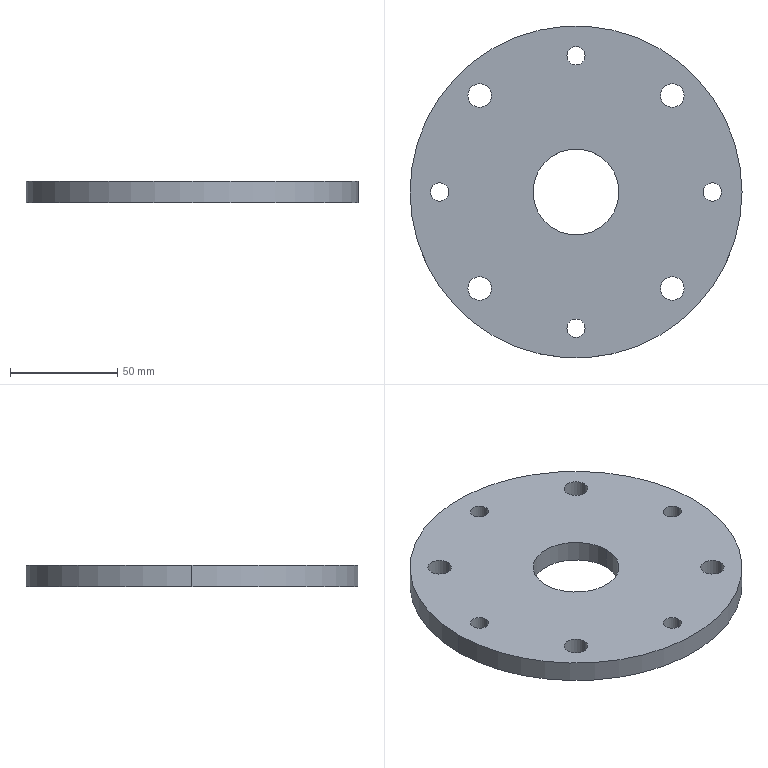Part | SolidWorks | features BaseBody 1, ICE 1 | 1 solid | 22 faces | box 155 x 155 x 10 mm | volume 169991 mm3 | cylinder 20 | plane 2 | commonest cylinder face diameters 8.5 x8 11 x8 40.1 x2 155 x2
STEP:
#1=CARTESIAN_POINT('',(20.05,0.,0.));
#2=VERTEX_POINT('',#1);
#3=CARTESIAN_POINT('',(-20.05,0.,0.));
#4=VERTEX_POINT('',#3);
#5=CARTESIAN_POINT('',(0.,0.,0.));
#6=DIRECTION('',(0.,0.,-1.));
#7=DIRECTION('',(0.,-1.,0.));
#8=AXIS2_PLACEMENT_3D('',#5,#6,#7);
#9=CIRCLE('',#8,20.05);
#10=EDGE_CURVE('',#2,#4,#9,.T.);
#11=ORIENTED_EDGE('',*,*,#10,.T.);
#12=CARTESIAN_POINT('',(-20.05,0.,10.));
#13=VERTEX_POINT('',#12);
#14=CARTESIAN_POINT('',(-20.05,0.,-0.001));
#15=DIRECTION('',(0.,0.,1.));
#16=VECTOR('',#15,1000.);
#17=LINE('',#14,#16);
#18=EDGE_CURVE('',#4,#13,#17,.T.);
#19=ORIENTED_EDGE('',*,*,#18,.T.);
#20=CARTESIAN_POINT('',(20.05,0.,10.));
#21=VERTEX_POINT('',#20);
#22=CARTESIAN_POINT('',(0.,0.,10.));
#23=DIRECTION('',(0.,0.,1.));
#24=DIRECTION('',(1.,0.,0.));
#25=AXIS2_PLACEMENT_3D('',#22,#23,#24);
#26=CIRCLE('',#25,20.05);
#27=EDGE_CURVE('',#13,#21,#26,.T.);
#28=ORIENTED_EDGE('',*,*,#27,.T.);
#29=CARTESIAN_POINT('',(20.05,0.,-0.001));
#30=DIRECTION('',(0.,0.,1.));
#31=VECTOR('',#30,1000.);
#32=LINE('',#29,#31);
#33=EDGE_CURVE('',#2,#21,#32,.T.);
#34=ORIENTED_EDGE('',*,*,#33,.F.);
#35=EDGE_LOOP('',(#11,#19,#28,#34));
#36=FACE_OUTER_BOUND('',#35,.T.);
#37=CARTESIAN_POINT('',(0.,0.,-0.001));
#38=DIRECTION('',(0.,0.,1.));
#39=DIRECTION('',(1.,0.,0.));
#40=AXIS2_PLACEMENT_3D('',#37,#38,#39);
#41=CYLINDRICAL_SURFACE('',#40,20.05);
#42=ADVANCED_FACE('',(#36),#41,.F.);
#43=CARTESIAN_POINT('',(-4.25,63.64,0.));
#44=VERTEX_POINT('',#43);
#45=CARTESIAN_POINT('',(4.25,63.64,0.));
#46=VERTEX_POINT('',#45);
#47=CARTESIAN_POINT('',(0.,63.64,0.));
#48=DIRECTION('',(0.,0.,1.));
#49=DIRECTION('',(1.,0.,0.));
#50=AXIS2_PLACEMENT_3D('',#47,#48,#49);
#51=CIRCLE('',#50,4.25);
#52=EDGE_CURVE('',#44,#46,#51,.T.);
#53=ORIENTED_EDGE('',*,*,#52,.F.);
#54=CARTESIAN_POINT('',(-4.25,63.64,10.));
#55=VERTEX_POINT('',#54);
#56=CARTESIAN_POINT('',(-4.25,63.64,10.));
#57=DIRECTION('',(0.,0.,1.));
#58=VECTOR('',#57,1000.);
#59=LINE('',#56,#58);
#60=EDGE_CURVE('',#44,#55,#59,.T.);
#61=ORIENTED_EDGE('',*,*,#60,.T.);
#62=CARTESIAN_POINT('',(4.25,63.64,10.));
#63=VERTEX_POINT('',#62);
#64=CARTESIAN_POINT('',(0.,63.64,10.));
#65=DIRECTION('',(0.,0.,1.));
#66=DIRECTION('',(1.,0.,0.));
#67=AXIS2_PLACEMENT_3D('',#64,#65,#66);
#68=CIRCLE('',#67,4.25);
#69=EDGE_CURVE('',#55,#63,#68,.T.);
#70=ORIENTED_EDGE('',*,*,#69,.T.);
#71=CARTESIAN_POINT('',(4.25,63.64,10.));
#72=DIRECTION('',(0.,0.,1.));
#73=VECTOR('',#72,1000.);
#74=LINE('',#71,#73);
#75=EDGE_CURVE('',#46,#63,#74,.T.);
#76=ORIENTED_EDGE('',*,*,#75,.F.);
#77=EDGE_LOOP('',(#53,#61,#70,#76));
#78=FACE_OUTER_BOUND('',#77,.T.);
#79=CARTESIAN_POINT('',(0.,63.64,10.));
#80=DIRECTION('',(0.,0.,1.));
#81=DIRECTION('',(1.,0.,0.));
#82=AXIS2_PLACEMENT_3D('',#79,#80,#81);
#83=CYLINDRICAL_SURFACE('',#82,4.25);
#84=ADVANCED_FACE('',(#78),#83,.F.);
#85=CARTESIAN_POINT('',(-67.89,0.,0.));
#86=VERTEX_POINT('',#85);
#87=CARTESIAN_POINT('',(-59.39,0.,0.));
#88=VERTEX_POINT('',#87);
#89=CARTESIAN_POINT('',(-63.64,0.,0.));
#90=DIRECTION('',(0.,0.,1.));
#91=DIRECTION('',(1.,0.,0.));
#92=AXIS2_PLACEMENT_3D('',#89,#90,#91);
#93=CIRCLE('',#92,4.25);
#94=EDGE_CURVE('',#86,#88,#93,.T.);
#95=ORIENTED_EDGE('',*,*,#94,.F.);
#96=CARTESIAN_POINT('',(-67.89,0.,10.));
#97=VERTEX_POINT('',#96);
#98=CARTESIAN_POINT('',(-67.89,0.,10.));
#99=DIRECTION('',(0.,0.,1.));
#100=VECTOR('',#99,1000.);
#101=LINE('',#98,#100);
#102=EDGE_CURVE('',#86,#97,#101,.T.);
#103=ORIENTED_EDGE('',*,*,#102,.T.);
#104=CARTESIAN_POINT('',(-59.39,0.,10.));
#105=VERTEX_POINT('',#104);
#106=CARTESIAN_POINT('',(-63.64,0.,10.));
#107=DIRECTION('',(0.,0.,1.));
#108=DIRECTION('',(1.,0.,0.));
#109=AXIS2_PLACEMENT_3D('',#106,#107,#108);
#110=CIRCLE('',#109,4.25);
#111=EDGE_CURVE('',#97,#105,#110,.T.);
#112=ORIENTED_EDGE('',*,*,#111,.T.);
#113=CARTESIAN_POINT('',(-59.39,0.,10.));
#114=DIRECTION('',(0.,0.,1.));
#115=VECTOR('',#114,1000.);
#116=LINE('',#113,#115);
#117=EDGE_CURVE('',#88,#105,#116,.T.);
#118=ORIENTED_EDGE('',*,*,#117,.F.);
#119=EDGE_LOOP('',(#95,#103,#112,#118));
#120=FACE_OUTER_BOUND('',#119,.T.);
#121=CARTESIAN_POINT('',(-63.64,0.,10.));
#122=DIRECTION('',(0.,0.,1.));
#123=DIRECTION('',(1.,0.,0.));
#124=AXIS2_PLACEMENT_3D('',#121,#122,#123);
#125=CYLINDRICAL_SURFACE('',#124,4.25);
#126=ADVANCED_FACE('',(#120),#125,.F.);
#127=CARTESIAN_POINT('',(-4.25,-63.64,0.));
#128=VERTEX_POINT('',#127);
#129=CARTESIAN_POINT('',(4.25,-63.64,0.));
#130=VERTEX_POINT('',#129);
#131=CARTESIAN_POINT('',(0.,-63.64,0.));
#132=DIRECTION('',(0.,0.,1.));
#133=DIRECTION('',(1.,0.,0.));
#134=AXIS2_PLACEMENT_3D('',#131,#132,#133);
#135=CIRCLE('',#134,4.25);
#136=EDGE_CURVE('',#128,#130,#135,.T.);
#137=ORIENTED_EDGE('',*,*,#136,.F.);
#138=CARTESIAN_POINT('',(-4.25,-63.64,10.));
#139=VERTEX_POINT('',#138);
#140=CARTESIAN_POINT('',(-4.25,-63.64,10.));
#141=DIRECTION('',(0.,0.,1.));
#142=VECTOR('',#141,1000.);
#143=LINE('',#140,#142);
#144=EDGE_CURVE('',#128,#139,#143,.T.);
#145=ORIENTED_EDGE('',*,*,#144,.T.);
#146=CARTESIAN_POINT('',(4.25,-63.64,10.));
#147=VERTEX_POINT('',#146);
#148=CARTESIAN_POINT('',(0.,-63.64,10.));
#149=DIRECTION('',(0.,0.,1.));
#150=DIRECTION('',(1.,0.,0.));
#151=AXIS2_PLACEMENT_3D('',#148,#149,#150);
#152=CIRCLE('',#151,4.25);
#153=EDGE_CURVE('',#139,#147,#152,.T.);
#154=ORIENTED_EDGE('',*,*,#153,.T.);
#155=CARTESIAN_POINT('',(4.25,-63.64,10.));
#156=DIRECTION('',(0.,0.,1.));
#157=VECTOR('',#156,1000.);
#158=LINE('',#155,#157);
#159=EDGE_CURVE('',#130,#147,#158,.T.);
#160=ORIENTED_EDGE('',*,*,#159,.F.);
#161=EDGE_LOOP('',(#137,#145,#154,#160));
#162=FACE_OUTER_BOUND('',#161,.T.);
#163=CARTESIAN_POINT('',(0.,-63.64,10.));
#164=DIRECTION('',(0.,0.,1.));
#165=DIRECTION('',(1.,0.,0.));
#166=AXIS2_PLACEMENT_3D('',#163,#164,#165);
#167=CYLINDRICAL_SURFACE('',#166,4.25);
#168=ADVANCED_FACE('',(#162),#167,.F.);
#169=CARTESIAN_POINT('',(59.39,0.,0.));
#170=VERTEX_POINT('',#169);
#171=CARTESIAN_POINT('',(67.89,0.,0.));
#172=VERTEX_POINT('',#171);
#173=CARTESIAN_POINT('',(63.64,0.,0.));
#174=DIRECTION('',(0.,0.,1.));
#175=DIRECTION('',(1.,0.,0.));
#176=AXIS2_PLACEMENT_3D('',#173,#174,#175);
#177=CIRCLE('',#176,4.25);
#178=EDGE_CURVE('',#170,#172,#177,.T.);
#179=ORIENTED_EDGE('',*,*,#178,.F.);
#180=CARTESIAN_POINT('',(59.39,0.,10.));
#181=VERTEX_POINT('',#180);
#182=CARTESIAN_POINT('',(59.39,0.,10.));
#183=DIRECTION('',(0.,0.,1.));
#184=VECTOR('',#183,1000.);
#185=LINE('',#182,#184);
#186=EDGE_CURVE('',#170,#181,#185,.T.);
#187=ORIENTED_EDGE('',*,*,#186,.T.);
#188=CARTESIAN_POINT('',(67.89,0.,10.));
#189=VERTEX_POINT('',#188);
#190=CARTESIAN_POINT('',(63.64,0.,10.));
#191=DIRECTION('',(0.,0.,1.));
#192=DIRECTION('',(1.,0.,0.));
#193=AXIS2_PLACEMENT_3D('',#190,#191,#192);
#194=CIRCLE('',#193,4.25);
#195=EDGE_CURVE('',#181,#189,#194,.T.);
#196=ORIENTED_EDGE('',*,*,#195,.T.);
#197=CARTESIAN_POINT('',(67.89,0.,10.));
#198=DIRECTION('',(0.,0.,1.));
#199=VECTOR('',#198,1000.);
#200=LINE('',#197,#199);
#201=EDGE_CURVE('',#172,#189,#200,.T.);
#202=ORIENTED_EDGE('',*,*,#201,.F.);
#203=EDGE_LOOP('',(#179,#187,#196,#202));
#204=FACE_OUTER_BOUND('',#203,.T.);
#205=CARTESIAN_POINT('',(63.64,0.,10.));
#206=DIRECTION('',(0.,0.,1.));
#207=DIRECTION('',(1.,0.,0.));
#208=AXIS2_PLACEMENT_3D('',#205,#206,#207);
#209=CYLINDRICAL_SURFACE('',#208,4.25);
#210=ADVANCED_FACE('',(#204),#209,.F.);
#211=CARTESIAN_POINT('',(-50.5,45.,0.));
#212=VERTEX_POINT('',#211);
#213=CARTESIAN_POINT('',(-39.5,45.,0.));
#214=VERTEX_POINT('',#213);
#215=CARTESIAN_POINT('',(-45.,45.,0.));
#216=DIRECTION('',(0.,0.,1.));
#217=DIRECTION('',(1.,0.,0.));
#218=AXIS2_PLACEMENT_3D('',#215,#216,#217);
#219=CIRCLE('',#218,5.5);
#220=EDGE_CURVE('',#212,#214,#219,.T.);
#221=ORIENTED_EDGE('',*,*,#220,.F.);
#222=CARTESIAN_POINT('',(-50.5,45.,10.));
#223=VERTEX_POINT('',#222);
#224=CARTESIAN_POINT('',(-50.5,45.,10.));
#225=DIRECTION('',(0.,0.,1.));
#226=VECTOR('',#225,1000.);
#227=LINE('',#224,#226);
#228=EDGE_CURVE('',#212,#223,#227,.T.);
#229=ORIENTED_EDGE('',*,*,#228,.T.);
#230=CARTESIAN_POINT('',(-39.5,45.,10.));
#231=VERTEX_POINT('',#230);
#232=CARTESIAN_POINT('',(-45.,45.,10.));
#233=DIRECTION('',(0.,0.,1.));
#234=DIRECTION('',(1.,0.,0.));
#235=AXIS2_PLACEMENT_3D('',#232,#233,#234);
#236=CIRCLE('',#235,5.5);
#237=EDGE_CURVE('',#223,#231,#236,.T.);
#238=ORIENTED_EDGE('',*,*,#237,.T.);
#239=CARTESIAN_POINT('',(-39.5,45.,10.));
#240=DIRECTION('',(0.,0.,1.));
#241=VECTOR('',#240,1000.);
#242=LINE('',#239,#241);
#243=EDGE_CURVE('',#214,#231,#242,.T.);
#244=ORIENTED_EDGE('',*,*,#243,.F.);
#245=EDGE_LOOP('',(#221,#229,#238,#244));
#246=FACE_OUTER_BOUND('',#245,.T.);
#247=CARTESIAN_POINT('',(-45.,45.,10.));
#248=DIRECTION('',(0.,0.,1.));
#249=DIRECTION('',(1.,0.,0.));
#250=AXIS2_PLACEMENT_3D('',#247,#248,#249);
#251=CYLINDRICAL_SURFACE('',#250,5.5);
#252=ADVANCED_FACE('',(#246),#251,.F.);
#253=CARTESIAN_POINT('',(39.5,45.,0.));
#254=VERTEX_POINT('',#253);
#255=CARTESIAN_POINT('',(50.5,45.,0.));
#256=VERTEX_POINT('',#255);
#257=CARTESIAN_POINT('',(45.,45.,0.));
#258=DIRECTION('',(0.,0.,1.));
#259=DIRECTION('',(1.,0.,0.));
#260=AXIS2_PLACEMENT_3D('',#257,#258,#259);
#261=CIRCLE('',#260,5.5);
#262=EDGE_CURVE('',#254,#256,#261,.T.);
#263=ORIENTED_EDGE('',*,*,#262,.F.);
#264=CARTESIAN_POINT('',(39.5,45.,10.));
#265=VERTEX_POINT('',#264);
#266=CARTESIAN_POINT('',(39.5,45.,10.));
#267=DIRECTION('',(0.,0.,1.));
#268=VECTOR('',#267,1000.);
#269=LINE('',#266,#268);
#270=EDGE_CURVE('',#254,#265,#269,.T.);
#271=ORIENTED_EDGE('',*,*,#270,.T.);
#272=CARTESIAN_POINT('',(50.5,45.,10.));
#273=VERTEX_POINT('',#272);
#274=CARTESIAN_POINT('',(45.,45.,10.));
#275=DIRECTION('',(0.,0.,1.));
#276=DIRECTION('',(1.,0.,0.));
#277=AXIS2_PLACEMENT_3D('',#274,#275,#276);
#278=CIRCLE('',#277,5.5);
#279=EDGE_CURVE('',#265,#273,#278,.T.);
#280=ORIENTED_EDGE('',*,*,#279,.T.);
#281=CARTESIAN_POINT('',(50.5,45.,10.));
#282=DIRECTION('',(0.,0.,1.));
#283=VECTOR('',#282,1000.);
#284=LINE('',#281,#283);
#285=EDGE_CURVE('',#256,#273,#284,.T.);
#286=ORIENTED_EDGE('',*,*,#285,.F.);
#287=EDGE_LOOP('',(#263,#271,#280,#286));
#288=FACE_OUTER_BOUND('',#287,.T.);
#289=CARTESIAN_POINT('',(45.,45.,10.));
#290=DIRECTION('',(0.,0.,1.));
#291=DIRECTION('',(1.,0.,0.));
#292=AXIS2_PLACEMENT_3D('',#289,#290,#291);
#293=CYLINDRICAL_SURFACE('',#292,5.5);
#294=ADVANCED_FACE('',(#288),#293,.F.);
#295=CARTESIAN_POINT('',(39.5,-45.,0.));
#296=VERTEX_POINT('',#295);
#297=CARTESIAN_POINT('',(50.5,-45.,0.));
#298=VERTEX_POINT('',#297);
#299=CARTESIAN_POINT('',(45.,-45.,0.));
#300=DIRECTION('',(0.,0.,1.));
#301=DIRECTION('',(1.,0.,0.));
#302=AXIS2_PLACEMENT_3D('',#299,#300,#301);
#303=CIRCLE('',#302,5.5);
#304=EDGE_CURVE('',#296,#298,#303,.T.);
#305=ORIENTED_EDGE('',*,*,#304,.F.);
#306=CARTESIAN_POINT('',(39.5,-45.,10.));
#307=VERTEX_POINT('',#306);
#308=CARTESIAN_POINT('',(39.5,-45.,10.));
#309=DIRECTION('',(0.,0.,1.));
#310=VECTOR('',#309,1000.);
#311=LINE('',#308,#310);
#312=EDGE_CURVE('',#296,#307,#311,.T.);
#313=ORIENTED_EDGE('',*,*,#312,.T.);
#314=CARTESIAN_POINT('',(50.5,-45.,10.));
#315=VERTEX_POINT('',#314);
#316=CARTESIAN_POINT('',(45.,-45.,10.));
#317=DIRECTION('',(0.,0.,1.));
#318=DIRECTION('',(1.,0.,0.));
#319=AXIS2_PLACEMENT_3D('',#316,#317,#318);
#320=CIRCLE('',#319,5.5);
#321=EDGE_CURVE('',#307,#315,#320,.T.);
#322=ORIENTED_EDGE('',*,*,#321,.T.);
#323=CARTESIAN_POINT('',(50.5,-45.,10.));
#324=DIRECTION('',(0.,0.,1.));
#325=VECTOR('',#324,1000.);
#326=LINE('',#323,#325);
#327=EDGE_CURVE('',#298,#315,#326,.T.);
#328=ORIENTED_EDGE('',*,*,#327,.F.);
#329=EDGE_LOOP('',(#305,#313,#322,#328));
#330=FACE_OUTER_BOUND('',#329,.T.);
#331=CARTESIAN_POINT('',(45.,-45.,10.));
#332=DIRECTION('',(0.,0.,1.));
#333=DIRECTION('',(1.,0.,0.));
#334=AXIS2_PLACEMENT_3D('',#331,#332,#333);
#335=CYLINDRICAL_SURFACE('',#334,5.5);
#336=ADVANCED_FACE('',(#330),#335,.F.);
#337=CARTESIAN_POINT('',(-50.5,-45.,0.));
#338=VERTEX_POINT('',#337);
#339=CARTESIAN_POINT('',(-39.5,-45.,0.));
#340=VERTEX_POINT('',#339);
#341=CARTESIAN_POINT('',(-45.,-45.,0.));
#342=DIRECTION('',(0.,0.,1.));
#343=DIRECTION('',(1.,0.,0.));
#344=AXIS2_PLACEMENT_3D('',#341,#342,#343);
#345=CIRCLE('',#344,5.5);
#346=EDGE_CURVE('',#338,#340,#345,.T.);
#347=ORIENTED_EDGE('',*,*,#346,.F.);
#348=CARTESIAN_POINT('',(-50.5,-45.,10.));
#349=VERTEX_POINT('',#348);
#350=CARTESIAN_POINT('',(-50.5,-45.,10.));
#351=DIRECTION('',(0.,0.,1.));
#352=VECTOR('',#351,1000.);
#353=LINE('',#350,#352);
#354=EDGE_CURVE('',#338,#349,#353,.T.);
#355=ORIENTED_EDGE('',*,*,#354,.T.);
#356=CARTESIAN_POINT('',(-39.5,-45.,10.));
#357=VERTEX_POINT('',#356);
#358=CARTESIAN_POINT('',(-45.,-45.,10.));
#359=DIRECTION('',(0.,0.,1.));
#360=DIRECTION('',(1.,0.,0.));
#361=AXIS2_PLACEMENT_3D('',#358,#359,#360);
#362=CIRCLE('',#361,5.5);
#363=EDGE_CURVE('',#349,#357,#362,.T.);
#364=ORIENTED_EDGE('',*,*,#363,.T.);
#365=CARTESIAN_POINT('',(-39.5,-45.,10.));
#366=DIRECTION('',(0.,0.,1.));
#367=VECTOR('',#366,1000.);
#368=LINE('',#365,#367);
#369=EDGE_CURVE('',#340,#357,#368,.T.);
#370=ORIENTED_EDGE('',*,*,#369,.F.);
#371=EDGE_LOOP('',(#347,#355,#364,#370));
#372=FACE_OUTER_BOUND('',#371,.T.);
#373=CARTESIAN_POINT('',(-45.,-45.,10.));
#374=DIRECTION('',(0.,0.,1.));
#375=DIRECTION('',(1.,0.,0.));
#376=AXIS2_PLACEMENT_3D('',#373,#374,#375);
#377=CYLINDRICAL_SURFACE('',#376,5.5);
#378=ADVANCED_FACE('',(#372),#377,.F.);
#379=CARTESIAN_POINT('',(77.5,0.,10.));
#380=VERTEX_POINT('',#379);
#381=CARTESIAN_POINT('',(-77.5,0.,10.));
#382=VERTEX_POINT('',#381);
#383=CARTESIAN_POINT('',(0.,0.,10.));
#384=DIRECTION('',(0.,0.,1.));
#385=DIRECTION('',(1.,0.,0.));
#386=AXIS2_PLACEMENT_3D('',#383,#384,#385);
#387=CIRCLE('',#386,77.5);
#388=EDGE_CURVE('',#380,#382,#387,.T.);
#389=ORIENTED_EDGE('',*,*,#388,.F.);
#390=CARTESIAN_POINT('',(77.5,0.,0.));
#391=VERTEX_POINT('',#390);
#392=CARTESIAN_POINT('',(77.5,0.,10.));
#393=DIRECTION('',(0.,0.,-1.));
#394=VECTOR('',#393,1000.);
#395=LINE('',#392,#394);
#396=EDGE_CURVE('',#380,#391,#395,.T.);
#397=ORIENTED_EDGE('',*,*,#396,.T.);
#398=CARTESIAN_POINT('',(-77.5,0.,0.));
#399=VERTEX_POINT('',#398);
#400=CARTESIAN_POINT('',(0.,0.,0.));
#401=DIRECTION('',(0.,0.,1.));
#402=DIRECTION('',(1.,0.,0.));
#403=AXIS2_PLACEMENT_3D('',#400,#401,#402);
#404=CIRCLE('',#403,77.5);
#405=EDGE_CURVE('',#391,#399,#404,.T.);
#406=ORIENTED_EDGE('',*,*,#405,.T.);
#407=CARTESIAN_POINT('',(-77.5,0.,10.));
#408=DIRECTION('',(0.,0.,-1.));
#409=VECTOR('',#408,1000.);
#410=LINE('',#407,#409);
#411=EDGE_CURVE('',#382,#399,#410,.T.);
#412=ORIENTED_EDGE('',*,*,#411,.F.);
#413=EDGE_LOOP('',(#389,#397,#406,#412));
#414=FACE_OUTER_BOUND('',#413,.T.);
#415=CARTESIAN_POINT('',(0.,0.,10.));
#416=DIRECTION('',(0.,0.,-1.));
#417=DIRECTION('',(-1.,0.,0.));
#418=AXIS2_PLACEMENT_3D('',#415,#416,#417);
#419=CYLINDRICAL_SURFACE('',#418,77.5);
#420=ADVANCED_FACE('',(#414),#419,.T.);
#421=ORIENTED_EDGE('',*,*,#10,.F.);
#422=CARTESIAN_POINT('',(0.,0.,0.));
#423=DIRECTION('',(0.,0.,-1.));
#424=DIRECTION('',(0.,-1.,0.));
#425=AXIS2_PLACEMENT_3D('',#422,#423,#424);
#426=CIRCLE('',#425,20.05);
#427=EDGE_CURVE('',#4,#2,#426,.T.);
#428=ORIENTED_EDGE('',*,*,#427,.F.);
#429=EDGE_LOOP('',(#421,#428));
#430=FACE_BOUND('',#429,.T.);
#431=CARTESIAN_POINT('',(-45.,-45.,0.));
#432=DIRECTION('',(0.,0.,1.));
#433=DIRECTION('',(1.,0.,0.));
#434=AXIS2_PLACEMENT_3D('',#431,#432,#433);
#435=CIRCLE('',#434,5.5);
#436=EDGE_CURVE('',#340,#338,#435,.T.);
#437=ORIENTED_EDGE('',*,*,#436,.T.);
#438=ORIENTED_EDGE('',*,*,#346,.T.);
#439=EDGE_LOOP('',(#437,#438));
#440=FACE_BOUND('',#439,.T.);
#441=CARTESIAN_POINT('',(45.,-45.,0.));
#442=DIRECTION('',(0.,0.,1.));
#443=DIRECTION('',(1.,0.,0.));
#444=AXIS2_PLACEMENT_3D('',#441,#442,#443);
#445=CIRCLE('',#444,5.5);
#446=EDGE_CURVE('',#298,#296,#445,.T.);
#447=ORIENTED_EDGE('',*,*,#446,.T.);
#448=ORIENTED_EDGE('',*,*,#304,.T.);
#449=EDGE_LOOP('',(#447,#448));
#450=FACE_BOUND('',#449,.T.);
#451=CARTESIAN_POINT('',(45.,45.,0.));
#452=DIRECTION('',(0.,0.,1.));
#453=DIRECTION('',(1.,0.,0.));
#454=AXIS2_PLACEMENT_3D('',#451,#452,#453);
#455=CIRCLE('',#454,5.5);
#456=EDGE_CURVE('',#256,#254,#455,.T.);
#457=ORIENTED_EDGE('',*,*,#456,.T.);
#458=ORIENTED_EDGE('',*,*,#262,.T.);
#459=EDGE_LOOP('',(#457,#458));
#460=FACE_BOUND('',#459,.T.);
#461=CARTESIAN_POINT('',(-45.,45.,0.));
#462=DIRECTION('',(0.,0.,1.));
#463=DIRECTION('',(1.,0.,0.));
#464=AXIS2_PLACEMENT_3D('',#461,#462,#463);
#465=CIRCLE('',#464,5.5);
#466=EDGE_CURVE('',#214,#212,#465,.T.);
#467=ORIENTED_EDGE('',*,*,#466,.T.);
#468=ORIENTED_EDGE('',*,*,#220,.T.);
#469=EDGE_LOOP('',(#467,#468));
#470=FACE_BOUND('',#469,.T.);
#471=CARTESIAN_POINT('',(63.64,0.,0.));
#472=DIRECTION('',(0.,0.,1.));
#473=DIRECTION('',(1.,0.,0.));
#474=AXIS2_PLACEMENT_3D('',#471,#472,#473);
#475=CIRCLE('',#474,4.25);
#476=EDGE_CURVE('',#172,#170,#475,.T.);
#477=ORIENTED_EDGE('',*,*,#476,.T.);
#478=ORIENTED_EDGE('',*,*,#178,.T.);
#479=EDGE_LOOP('',(#477,#478));
#480=FACE_BOUND('',#479,.T.);
#481=CARTESIAN_POINT('',(0.,-63.64,0.));
#482=DIRECTION('',(0.,0.,1.));
#483=DIRECTION('',(1.,0.,0.));
#484=AXIS2_PLACEMENT_3D('',#481,#482,#483);
#485=CIRCLE('',#484,4.25);
#486=EDGE_CURVE('',#130,#128,#485,.T.);
#487=ORIENTED_EDGE('',*,*,#486,.T.);
#488=ORIENTED_EDGE('',*,*,#136,.T.);
#489=EDGE_LOOP('',(#487,#488));
#490=FACE_BOUND('',#489,.T.);
#491=CARTESIAN_POINT('',(-63.64,0.,0.));
#492=DIRECTION('',(0.,0.,1.));
#493=DIRECTION('',(1.,0.,0.));
#494=AXIS2_PLACEMENT_3D('',#491,#492,#493);
#495=CIRCLE('',#494,4.25);
#496=EDGE_CURVE('',#88,#86,#495,.T.);
#497=ORIENTED_EDGE('',*,*,#496,.T.);
#498=ORIENTED_EDGE('',*,*,#94,.T.);
#499=EDGE_LOOP('',(#497,#498));
#500=FACE_BOUND('',#499,.T.);
#501=CARTESIAN_POINT('',(0.,63.64,0.));
#502=DIRECTION('',(0.,0.,1.));
#503=DIRECTION('',(1.,0.,0.));
#504=AXIS2_PLACEMENT_3D('',#501,#502,#503);
#505=CIRCLE('',#504,4.25);
#506=EDGE_CURVE('',#46,#44,#505,.T.);
#507=ORIENTED_EDGE('',*,*,#506,.T.);
#508=ORIENTED_EDGE('',*,*,#52,.T.);
#509=EDGE_LOOP('',(#507,#508));
#510=FACE_BOUND('',#509,.T.);
#511=CARTESIAN_POINT('',(0.,0.,0.));
#512=DIRECTION('',(0.,0.,1.));
#513=DIRECTION('',(1.,0.,0.));
#514=AXIS2_PLACEMENT_3D('',#511,#512,#513);
#515=CIRCLE('',#514,77.5);
#516=EDGE_CURVE('',#399,#391,#515,.T.);
#517=ORIENTED_EDGE('',*,*,#516,.F.);
#518=ORIENTED_EDGE('',*,*,#405,.F.);
#519=EDGE_LOOP('',(#517,#518));
#520=FACE_OUTER_BOUND('',#519,.T.);
#521=CARTESIAN_POINT('',(0.,0.,0.));
#522=DIRECTION('',(0.,0.,1.));
#523=DIRECTION('',(0.,-1.,0.));
#524=AXIS2_PLACEMENT_3D('',#521,#522,#523);
#525=PLANE('',#524);
#526=ADVANCED_FACE('',(#430,#440,#450,#460,#470,#480,#490,#500,#510,#520),#525,.F.);
#527=CARTESIAN_POINT('',(0.,0.,10.));
#528=DIRECTION('',(0.,0.,1.));
#529=DIRECTION('',(1.,0.,0.));
#530=AXIS2_PLACEMENT_3D('',#527,#528,#529);
#531=CIRCLE('',#530,20.05);
#532=EDGE_CURVE('',#21,#13,#531,.T.);
#533=ORIENTED_EDGE('',*,*,#532,.F.);
#534=ORIENTED_EDGE('',*,*,#27,.F.);
#535=EDGE_LOOP('',(#533,#534));
#536=FACE_BOUND('',#535,.T.);
#537=CARTESIAN_POINT('',(-45.,-45.,10.));
#538=DIRECTION('',(0.,0.,1.));
#539=DIRECTION('',(1.,0.,0.));
#540=AXIS2_PLACEMENT_3D('',#537,#538,#539);
#541=CIRCLE('',#540,5.5);
#542=EDGE_CURVE('',#357,#349,#541,.T.);
#543=ORIENTED_EDGE('',*,*,#542,.F.);
#544=ORIENTED_EDGE('',*,*,#363,.F.);
#545=EDGE_LOOP('',(#543,#544));
#546=FACE_BOUND('',#545,.T.);
#547=CARTESIAN_POINT('',(45.,-45.,10.));
#548=DIRECTION('',(0.,0.,1.));
#549=DIRECTION('',(1.,0.,0.));
#550=AXIS2_PLACEMENT_3D('',#547,#548,#549);
#551=CIRCLE('',#550,5.5);
#552=EDGE_CURVE('',#315,#307,#551,.T.);
#553=ORIENTED_EDGE('',*,*,#552,.F.);
#554=ORIENTED_EDGE('',*,*,#321,.F.);
#555=EDGE_LOOP('',(#553,#554));
#556=FACE_BOUND('',#555,.T.);
#557=CARTESIAN_POINT('',(45.,45.,10.));
#558=DIRECTION('',(0.,0.,1.));
#559=DIRECTION('',(1.,0.,0.));
#560=AXIS2_PLACEMENT_3D('',#557,#558,#559);
#561=CIRCLE('',#560,5.5);
#562=EDGE_CURVE('',#273,#265,#561,.T.);
#563=ORIENTED_EDGE('',*,*,#562,.F.);
#564=ORIENTED_EDGE('',*,*,#279,.F.);
#565=EDGE_LOOP('',(#563,#564));
#566=FACE_BOUND('',#565,.T.);
#567=CARTESIAN_POINT('',(-45.,45.,10.));
#568=DIRECTION('',(0.,0.,1.));
#569=DIRECTION('',(1.,0.,0.));
#570=AXIS2_PLACEMENT_3D('',#567,#568,#569);
#571=CIRCLE('',#570,5.5);
#572=EDGE_CURVE('',#231,#223,#571,.T.);
#573=ORIENTED_EDGE('',*,*,#572,.F.);
#574=ORIENTED_EDGE('',*,*,#237,.F.);
#575=EDGE_LOOP('',(#573,#574));
#576=FACE_BOUND('',#575,.T.);
#577=CARTESIAN_POINT('',(63.64,0.,10.));
#578=DIRECTION('',(0.,0.,1.));
#579=DIRECTION('',(1.,0.,0.));
#580=AXIS2_PLACEMENT_3D('',#577,#578,#579);
#581=CIRCLE('',#580,4.25);
#582=EDGE_CURVE('',#189,#181,#581,.T.);
#583=ORIENTED_EDGE('',*,*,#582,.F.);
#584=ORIENTED_EDGE('',*,*,#195,.F.);
#585=EDGE_LOOP('',(#583,#584));
#586=FACE_BOUND('',#585,.T.);
#587=CARTESIAN_POINT('',(0.,-63.64,10.));
#588=DIRECTION('',(0.,0.,1.));
#589=DIRECTION('',(1.,0.,0.));
#590=AXIS2_PLACEMENT_3D('',#587,#588,#589);
#591=CIRCLE('',#590,4.25);
#592=EDGE_CURVE('',#147,#139,#591,.T.);
#593=ORIENTED_EDGE('',*,*,#592,.F.);
#594=ORIENTED_EDGE('',*,*,#153,.F.);
#595=EDGE_LOOP('',(#593,#594));
#596=FACE_BOUND('',#595,.T.);
#597=CARTESIAN_POINT('',(-63.64,0.,10.));
#598=DIRECTION('',(0.,0.,1.));
#599=DIRECTION('',(1.,0.,0.));
#600=AXIS2_PLACEMENT_3D('',#597,#598,#599);
#601=CIRCLE('',#600,4.25);
#602=EDGE_CURVE('',#105,#97,#601,.T.);
#603=ORIENTED_EDGE('',*,*,#602,.F.);
#604=ORIENTED_EDGE('',*,*,#111,.F.);
#605=EDGE_LOOP('',(#603,#604));
#606=FACE_BOUND('',#605,.T.);
#607=CARTESIAN_POINT('',(0.,63.64,10.));
#608=DIRECTION('',(0.,0.,1.));
#609=DIRECTION('',(1.,0.,0.));
#610=AXIS2_PLACEMENT_3D('',#607,#608,#609);
#611=CIRCLE('',#610,4.25);
#612=EDGE_CURVE('',#63,#55,#611,.T.);
#613=ORIENTED_EDGE('',*,*,#612,.F.);
#614=ORIENTED_EDGE('',*,*,#69,.F.);
#615=EDGE_LOOP('',(#613,#614));
#616=FACE_BOUND('',#615,.T.);
#617=CARTESIAN_POINT('',(0.,0.,10.));
#618=DIRECTION('',(0.,0.,1.));
#619=DIRECTION('',(1.,0.,0.));
#620=AXIS2_PLACEMENT_3D('',#617,#618,#619);
#621=CIRCLE('',#620,77.5);
#622=EDGE_CURVE('',#382,#380,#621,.T.);
#623=ORIENTED_EDGE('',*,*,#622,.T.);
#624=ORIENTED_EDGE('',*,*,#388,.T.);
#625=EDGE_LOOP('',(#623,#624));
#626=FACE_OUTER_BOUND('',#625,.T.);
#627=CARTESIAN_POINT('',(0.,0.,10.));
#628=DIRECTION('',(0.,0.,1.));
#629=DIRECTION('',(0.,-1.,0.));
#630=AXIS2_PLACEMENT_3D('',#627,#628,#629);
#631=PLANE('',#630);
#632=ADVANCED_FACE('',(#536,#546,#556,#566,#576,#586,#596,#606,#616,#626),#631,.T.);
#633=ORIENTED_EDGE('',*,*,#396,.F.);
#634=ORIENTED_EDGE('',*,*,#622,.F.);
#635=ORIENTED_EDGE('',*,*,#411,.T.);
#636=ORIENTED_EDGE('',*,*,#516,.T.);
#637=EDGE_LOOP('',(#633,#634,#635,#636));
#638=FACE_OUTER_BOUND('',#637,.T.);
#639=CARTESIAN_POINT('',(0.,0.,10.));
#640=DIRECTION('',(0.,0.,-1.));
#641=DIRECTION('',(-1.,0.,0.));
#642=AXIS2_PLACEMENT_3D('',#639,#640,#641);
#643=CYLINDRICAL_SURFACE('',#642,77.5);
#644=ADVANCED_FACE('',(#638),#643,.T.);
#645=ORIENTED_EDGE('',*,*,#354,.F.);
#646=ORIENTED_EDGE('',*,*,#436,.F.);
#647=ORIENTED_EDGE('',*,*,#369,.T.);
#648=ORIENTED_EDGE('',*,*,#542,.T.);
#649=EDGE_LOOP('',(#645,#646,#647,#648));
#650=FACE_OUTER_BOUND('',#649,.T.);
#651=CARTESIAN_POINT('',(-45.,-45.,10.));
#652=DIRECTION('',(0.,0.,1.));
#653=DIRECTION('',(1.,0.,0.));
#654=AXIS2_PLACEMENT_3D('',#651,#652,#653);
#655=CYLINDRICAL_SURFACE('',#654,5.5);
#656=ADVANCED_FACE('',(#650),#655,.F.);
#657=ORIENTED_EDGE('',*,*,#312,.F.);
#658=ORIENTED_EDGE('',*,*,#446,.F.);
#659=ORIENTED_EDGE('',*,*,#327,.T.);
#660=ORIENTED_EDGE('',*,*,#552,.T.);
#661=EDGE_LOOP('',(#657,#658,#659,#660));
#662=FACE_OUTER_BOUND('',#661,.T.);
#663=CARTESIAN_POINT('',(45.,-45.,10.));
#664=DIRECTION('',(0.,0.,1.));
#665=DIRECTION('',(1.,0.,0.));
#666=AXIS2_PLACEMENT_3D('',#663,#664,#665);
#667=CYLINDRICAL_SURFACE('',#666,5.5);
#668=ADVANCED_FACE('',(#662),#667,.F.);
#669=ORIENTED_EDGE('',*,*,#270,.F.);
#670=ORIENTED_EDGE('',*,*,#456,.F.);
#671=ORIENTED_EDGE('',*,*,#285,.T.);
#672=ORIENTED_EDGE('',*,*,#562,.T.);
#673=EDGE_LOOP('',(#669,#670,#671,#672));
#674=FACE_OUTER_BOUND('',#673,.T.);
#675=CARTESIAN_POINT('',(45.,45.,10.));
#676=DIRECTION('',(0.,0.,1.));
#677=DIRECTION('',(1.,0.,0.));
#678=AXIS2_PLACEMENT_3D('',#675,#676,#677);
#679=CYLINDRICAL_SURFACE('',#678,5.5);
#680=ADVANCED_FACE('',(#674),#679,.F.);
#681=ORIENTED_EDGE('',*,*,#228,.F.);
#682=ORIENTED_EDGE('',*,*,#466,.F.);
#683=ORIENTED_EDGE('',*,*,#243,.T.);
#684=ORIENTED_EDGE('',*,*,#572,.T.);
#685=EDGE_LOOP('',(#681,#682,#683,#684));
#686=FACE_OUTER_BOUND('',#685,.T.);
#687=CARTESIAN_POINT('',(-45.,45.,10.));
#688=DIRECTION('',(0.,0.,1.));
#689=DIRECTION('',(1.,0.,0.));
#690=AXIS2_PLACEMENT_3D('',#687,#688,#689);
#691=CYLINDRICAL_SURFACE('',#690,5.5);
#692=ADVANCED_FACE('',(#686),#691,.F.);
#693=ORIENTED_EDGE('',*,*,#186,.F.);
#694=ORIENTED_EDGE('',*,*,#476,.F.);
#695=ORIENTED_EDGE('',*,*,#201,.T.);
#696=ORIENTED_EDGE('',*,*,#582,.T.);
#697=EDGE_LOOP('',(#693,#694,#695,#696));
#698=FACE_OUTER_BOUND('',#697,.T.);
#699=CARTESIAN_POINT('',(63.64,0.,10.));
#700=DIRECTION('',(0.,0.,1.));
#701=DIRECTION('',(1.,0.,0.));
#702=AXIS2_PLACEMENT_3D('',#699,#700,#701);
#703=CYLINDRICAL_SURFACE('',#702,4.25);
#704=ADVANCED_FACE('',(#698),#703,.F.);
#705=ORIENTED_EDGE('',*,*,#144,.F.);
#706=ORIENTED_EDGE('',*,*,#486,.F.);
#707=ORIENTED_EDGE('',*,*,#159,.T.);
#708=ORIENTED_EDGE('',*,*,#592,.T.);
#709=EDGE_LOOP('',(#705,#706,#707,#708));
#710=FACE_OUTER_BOUND('',#709,.T.);
#711=CARTESIAN_POINT('',(0.,-63.64,10.));
#712=DIRECTION('',(0.,0.,1.));
#713=DIRECTION('',(1.,0.,0.));
#714=AXIS2_PLACEMENT_3D('',#711,#712,#713);
#715=CYLINDRICAL_SURFACE('',#714,4.25);
#716=ADVANCED_FACE('',(#710),#715,.F.);
#717=ORIENTED_EDGE('',*,*,#102,.F.);
#718=ORIENTED_EDGE('',*,*,#496,.F.);
#719=ORIENTED_EDGE('',*,*,#117,.T.);
#720=ORIENTED_EDGE('',*,*,#602,.T.);
#721=EDGE_LOOP('',(#717,#718,#719,#720));
#722=FACE_OUTER_BOUND('',#721,.T.);
#723=CARTESIAN_POINT('',(-63.64,0.,10.));
#724=DIRECTION('',(0.,0.,1.));
#725=DIRECTION('',(1.,0.,0.));
#726=AXIS2_PLACEMENT_3D('',#723,#724,#725);
#727=CYLINDRICAL_SURFACE('',#726,4.25);
#728=ADVANCED_FACE('',(#722),#727,.F.);
#729=ORIENTED_EDGE('',*,*,#60,.F.);
#730=ORIENTED_EDGE('',*,*,#506,.F.);
#731=ORIENTED_EDGE('',*,*,#75,.T.);
#732=ORIENTED_EDGE('',*,*,#612,.T.);
#733=EDGE_LOOP('',(#729,#730,#731,#732));
#734=FACE_OUTER_BOUND('',#733,.T.);
#735=CARTESIAN_POINT('',(0.,63.64,10.));
#736=DIRECTION('',(0.,0.,1.));
#737=DIRECTION('',(1.,0.,0.));
#738=AXIS2_PLACEMENT_3D('',#735,#736,#737);
#739=CYLINDRICAL_SURFACE('',#738,4.25);
#740=ADVANCED_FACE('',(#734),#739,.F.);
#741=ORIENTED_EDGE('',*,*,#18,.F.);
#742=ORIENTED_EDGE('',*,*,#427,.T.);
#743=ORIENTED_EDGE('',*,*,#33,.T.);
#744=ORIENTED_EDGE('',*,*,#532,.T.);
#745=EDGE_LOOP('',(#741,#742,#743,#744));
#746=FACE_OUTER_BOUND('',#745,.T.);
#747=CARTESIAN_POINT('',(0.,0.,-0.001));
#748=DIRECTION('',(0.,0.,1.));
#749=DIRECTION('',(1.,0.,0.));
#750=AXIS2_PLACEMENT_3D('',#747,#748,#749);
#751=CYLINDRICAL_SURFACE('',#750,20.05);
#752=ADVANCED_FACE('',(#746),#751,.F.);
#753=CLOSED_SHELL('',(#42,#84,#126,#168,#210,#252,#294,#336,#378,#420,#526,#632,#644,#656,#668,#680,#692,#704,#716,#728,#740,#752));
#754=MANIFOLD_SOLID_BREP('',#753);
#755=CARTESIAN_POINT('',(0.,0.,0.));
#756=DIRECTION('',(0.,0.,1.));
#757=DIRECTION('',(1.,0.,0.));
#758=AXIS2_PLACEMENT_3D('',#755,#756,#757);
#759=(LENGTH_UNIT()NAMED_UNIT(*)SI_UNIT(.MILLI.,.METRE.));
#760=UNCERTAINTY_MEASURE_WITH_UNIT(LENGTH_MEASURE(0.00001),#759,'','');
#761=(NAMED_UNIT(*)PLANE_ANGLE_UNIT()SI_UNIT($,.RADIAN.));
#762=(NAMED_UNIT(*)SI_UNIT($,.STERADIAN.)SOLID_ANGLE_UNIT());
#763=(GEOMETRIC_REPRESENTATION_CONTEXT(3)GLOBAL_UNCERTAINTY_ASSIGNED_CONTEXT((#760))GLOBAL_UNIT_ASSIGNED_CONTEXT((#759,#761,#762))REPRESENTATION_CONTEXT('',''));
#764=ADVANCED_BREP_SHAPE_REPRESENTATION('',(#754,#758),#763);